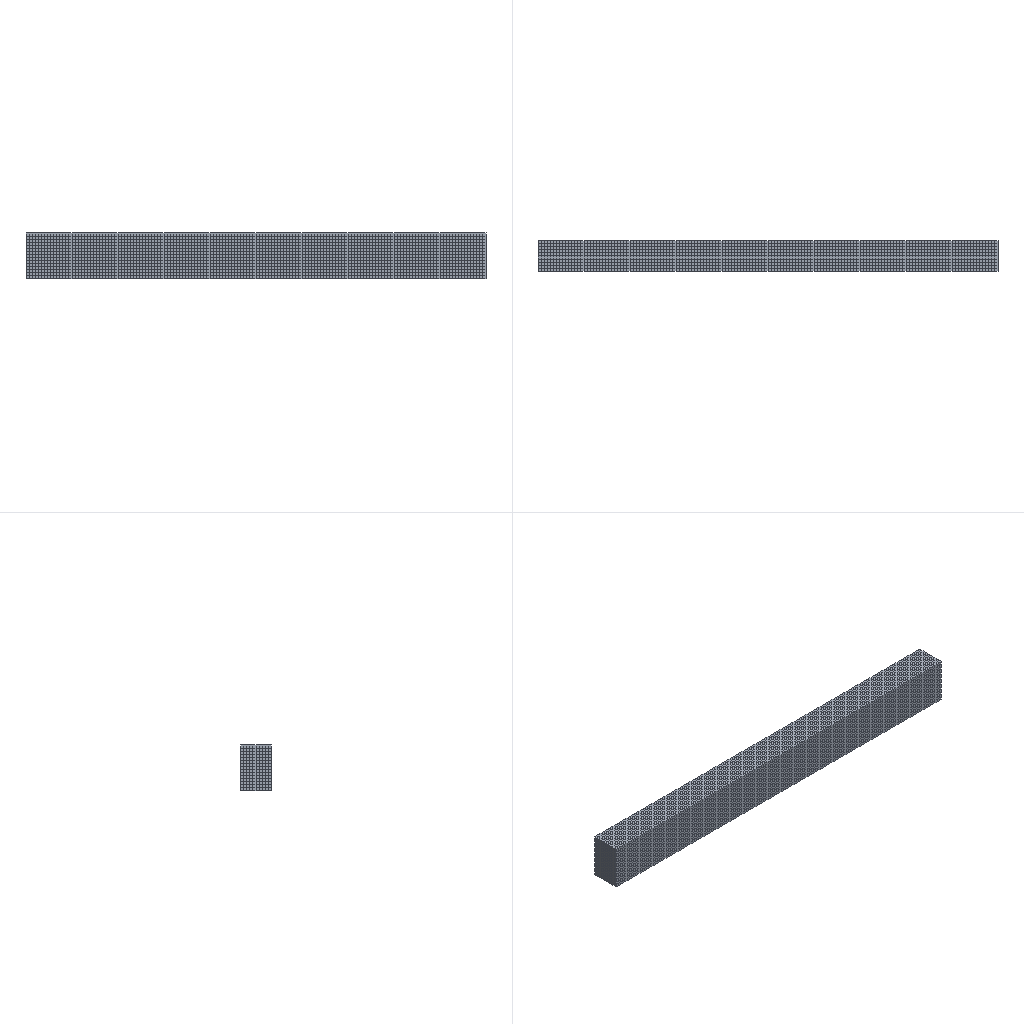Simulation study | abaqus
Set-up summary:
category,name,step,type,value,unit,region
solver,abaqus
solver,version,,,Abaqus/Explicit 3DEXPERIENCE R2017x
units,not stated in the deck,,not stated
analysis,deck,,transient,transient
load_step,Step-1,Step-1,transient
load_step,requested,,,1
mesh,nodes,,,27569
mesh,elements,,,23424
element_type,R3D4,,rigid,924
element_type,C3D8R,,solid,22500
load,load commands in deck,,count,1
bc,support commands in deck,,count,7
material,BAMBOO,,in results
check,setup vs results,,match,"per instance, exact: element labels, types and connectivity; labels of the nodes the elements use; coordinates of those nodes at SINGLE_PRECISION in 4 of 4 instance(s)"
Abaqus input file, long lists of numbers shortened:
*Heading
** Job name: Job-1 Model name: Job-1
** Generated by: Abaqus/CAE 2017
*Preprint, echo=NO, model=NO, history=NO, contact=NO
**
** PARTS
**
*Part, name=BAMBOO
*Node
      1,         150.,           0.,          30.
      2,         150.,          -2.,          30.
** (26574 more lines like these left out)
*Element, type=C3D8R
    1,     1,     2,   178,   177,    12,    13,   189,   188
    2,     2,     3,   179,   178,    13,    14,   190,   189
** (22498 more lines like these left out)
*Nset, nset=_PICKEDSET2, internal, generate
     1,  26576,      1
*Elset, elset=_PICKEDSET2, internal, generate
     1,  22500,      1
*Orientation, name=Ori-1
          1.,           0.,           0.,           0.,           1.,           0.
3, 0.
** Section: Section-1-_PICKEDSET2
*Solid Section, elset=_PICKEDSET2, orientation=Ori-1, material=BAMBOO
,
*End Part
**
*Part, name=STEEL
*Node
      1,   4.797,   -1.409,          20.
      2,   4.206,  -2.703,          20.
** (329 more lines like these left out)
*Element, type=R3D4
  1,  22,   1,  23,  44
  2,   1,   2,  24,  23
** (306 more lines like these left out)
*Nset, nset=STEEL-RefPt_, internal
 331,
*Nset, nset=STEEL-REFPT_, internal
 331,
*Elset, elset=STEEL, generate
   1,  308,    1
*End Part
**
**
** ASSEMBLY
**
*Assembly, name=Assembly
**
*Instance, name=BAMBOO-1, part=BAMBOO
*End Instance
**
*Instance, name=STEEL-1, part=STEEL
          0.,           0.,          -5.
          0.,           0.,          -5.,           1.,           0.,          -5.,          90.
*End Instance
**
*Instance, name=STEEL-1-LIN-2-1, part=STEEL
        120.,           0.,          35.
        120.,           0.,          35.,         121.,           0.,          35.,          90.
*End Instance
**
*Instance, name=STEEL-1-LIN-2-1-1, part=STEEL
       -120.,           0.,          35.
       -120.,           0.,          35.,        -119.,           0.,          35.,          90.
*End Instance
**
*Nset, nset=SET-4, instance=STEEL-1-LIN-2-1
 331,
*Nset, nset=SET-4, instance=STEEL-1-LIN-2-1-1
 331,
*Nset, nset=SET-5, instance=STEEL-1
 331,
*Nset, nset=_PickedSet13, internal, instance=STEEL-1-LIN-2-1
 331,
*Nset, nset=_PickedSet15, internal, instance=STEEL-1-LIN-2-1-1
 331,
** Constraint: RigidBody-1
*Rigid Body, ref node=STEEL-1.STEEL-REFPT_, elset=STEEL-1.STEEL
** Constraint: RigidBody-2
*Rigid Body, ref node=_PickedSet13, elset=STEEL-1-LIN-2-1.STEEL
** Constraint: RigidBody-3
*Rigid Body, ref node=_PickedSet15, elset=STEEL-1-LIN-2-1-1.STEEL
*End Assembly
*Amplitude, name=AMP-1, definition=SMOOTH STEP
             0.,              0.,            0.01,              1.
**
** MATERIALS
**
*Material, name=BAMBOO
*Density
 9.58e-10,
*Depvar, delete=1
      6,
*Elastic, type=ENGINEERING CONSTANTS
146000.,8010.,8010., 0.32, 0.32,  0.3,5060.,5060.
3860.,
*User Defined Field
**
** INTERACTION PROPERTIES
**
*Surface Interaction, name=INTPROP-1
*Friction
 0.4,
*Surface Behavior, pressure-overclosure=HARD
**
** BOUNDARY CONDITIONS
**
** Name: Disp-BC-1 Type: 对称/反对称/完全固定
*Boundary
SET-4, ENCASTRE
**
** INTERACTIONS
**
** Interaction: general_contact
*Contact, op=NEW
*Contact Inclusions, ALL EXTERIOR
*Contact Property Assignment
 ,  , INTPROP-1
** ----------------------------------------------------------------
**
** STEP: Step-1
**
*Step, name=Step-1, nlgeom=YES
*Dynamic, Explicit
, 0.01
*Bulk Viscosity
0.06, 1.2
** Mass Scaling: Semi-Automatic
**               Whole Model
*Fixed Mass Scaling, factor=500.
**
** BOUNDARY CONDITIONS
**
** Name: Disp-BC-2 Type: 位移/转角
*Boundary, amplitude=AMP-1
SET-5, 1, 1
** Name: Disp-BC-3 Type: 位移/转角
*Boundary, amplitude=AMP-1
SET-5, 2, 2
** Name: Disp-BC-4 Type: 位移/转角
*Boundary, amplitude=AMP-1
SET-5, 3, 3, 10.
** Name: Disp-BC-5 Type: 位移/转角
*Boundary, amplitude=AMP-1
SET-5, 4, 4
** Name: Disp-BC-6 Type: 位移/转角
*Boundary, amplitude=AMP-1
SET-5, 5, 5
** Name: Disp-BC-7 Type: 位移/转角
*Boundary, amplitude=AMP-1
SET-5, 6, 6
**
** OUTPUT REQUESTS
**
*Restart, write, number interval=1, time marks=NO
**
** FIELD OUTPUT: F-Output-1
**
*Output, field, number interval=50
*Node Output
A, CF, RF, RM, RT, U, V
*Element Output, directions=YES
E, LE, PE, PEEQ, PEEQMAX, PEEQT, PEEQVAVG, PEMAG, PEVAVG, VEEQ
**
** FIELD OUTPUT: F-Output-3
**
*Element Output, directions=YES
CTSHR, E, FV, MFR, MISES, MISESMAX, MISESONLY, S, SDV, SSAVG, STATUS, SVAVG, TSHR
*Contact Output
CDISP, CSTRESS
**
** HISTORY OUTPUT: H-Output-1
**
*Output, history, time interval=5e-05
*Node Output, nset=SET-5
RF3, U3
*End Step
Results summary:
result,step,Step-1,completed,increments=3365 time=0.01/0.01
result,analysis,,,transient
result,last_loadstep,,,1
result,primary field,,,U
result,reaction total,,FX,751.082,model units
result,reaction total,,FY,-1096.732,model units
result,reaction total,,FZ,-62859.023,model units